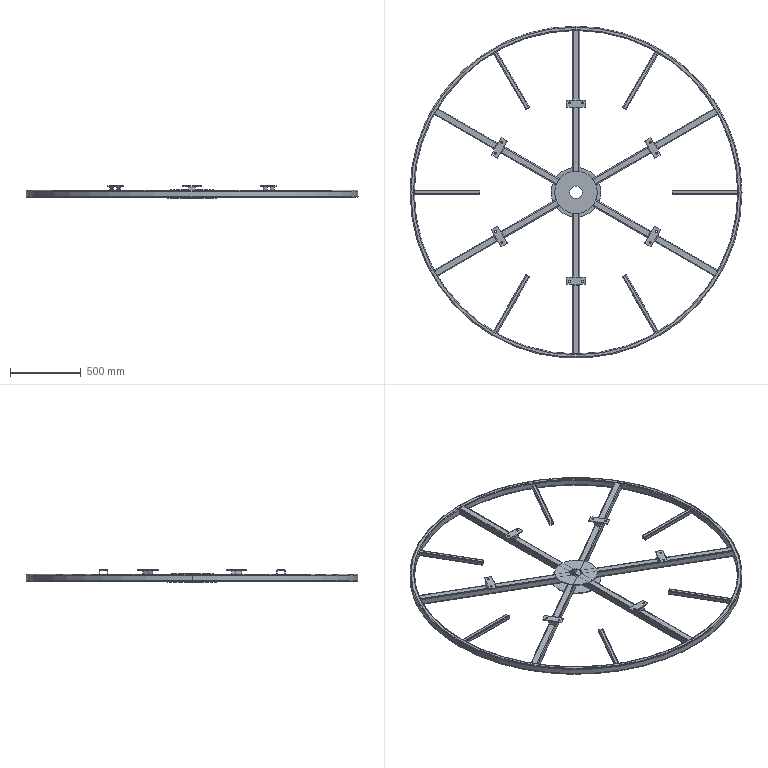Part | SolidWorks | features FlatPattern 6, ICE 5, WeldMemberFeat 3, CirPattern 2, HoleWzd 2, 3DProfileFeature 1, EdgeFlange 1, Fillet 1, SMBaseFlange 1, SheetMetal 1, WeldmentFeature 1 | 21 solids | 488 faces | box 2340 x 2340 x 85 mm | volume 8494790 mm3 | plane 258 | cylinder 176 | torus 30 | cone 24 | commonest cylinder face diameters 6 x48 12 x48 10 x24 14 x24 1.473 x12 11.473 x12